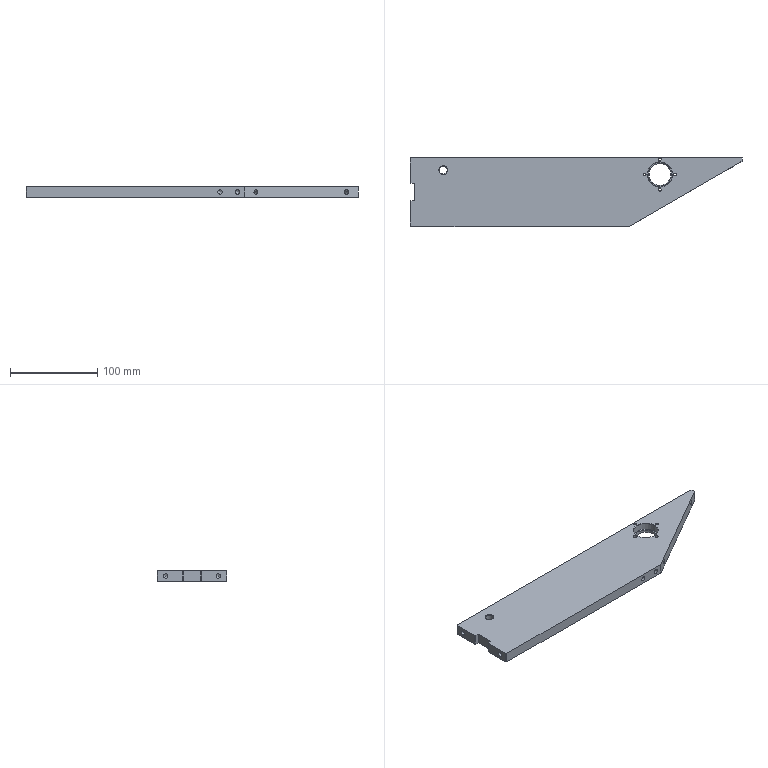Part | NX | 1 solid | 41 faces | box 380 x 80 x 12 mm | volume 295210 mm3 | plane 17 | cylinder 13 | cone 11 | commonest cylinder face diameters 5 x6 3.3 x4 9 x1 25 x1 28 x1
STEP:
#1=CARTESIAN_POINT('',(-190.,-32.5,-6.));
#2=VERTEX_POINT('',#1);
#3=CARTESIAN_POINT('',(-190.,-30.,-6.));
#4=DIRECTION('',(-1.,0.,0.));
#5=DIRECTION('',(0.,-1.,0.));
#6=AXIS2_PLACEMENT_3D('',#3,#4,#5);
#7=CIRCLE('',#6,2.5);
#8=EDGE_CURVE('',#2,#2,#7,.T.);
#9=ORIENTED_EDGE('',*,*,#8,.F.);
#10=EDGE_LOOP('',(#9));
#11=FACE_BOUND('',#10,.T.);
#12=CARTESIAN_POINT('',(-190.,-11.,0.));
#13=VERTEX_POINT('',#12);
#14=CARTESIAN_POINT('',(-190.,-39.,0.));
#15=VERTEX_POINT('',#14);
#16=CARTESIAN_POINT('',(-190.,40.,0.));
#17=DIRECTION('',(0.,-1.,0.));
#18=VECTOR('',#17,1000.);
#19=LINE('',#16,#18);
#20=EDGE_CURVE('',#13,#15,#19,.T.);
#21=ORIENTED_EDGE('',*,*,#20,.F.);
#22=CARTESIAN_POINT('',(-190.,-11.,-12.));
#23=VERTEX_POINT('',#22);
#24=CARTESIAN_POINT('',(-190.,-11.,0.));
#25=DIRECTION('',(0.,0.,-1.));
#26=VECTOR('',#25,1000.);
#27=LINE('',#24,#26);
#28=EDGE_CURVE('',#13,#23,#27,.T.);
#29=ORIENTED_EDGE('',*,*,#28,.T.);
#30=CARTESIAN_POINT('',(-190.,-39.,-12.));
#31=VERTEX_POINT('',#30);
#32=CARTESIAN_POINT('',(-190.,40.,-12.));
#33=DIRECTION('',(0.,-1.,0.));
#34=VECTOR('',#33,1000.);
#35=LINE('',#32,#34);
#36=EDGE_CURVE('',#23,#31,#35,.T.);
#37=ORIENTED_EDGE('',*,*,#36,.T.);
#38=CARTESIAN_POINT('',(-190.,-39.,0.));
#39=DIRECTION('',(0.,0.,1.));
#40=VECTOR('',#39,1000.);
#41=LINE('',#38,#40);
#42=EDGE_CURVE('',#31,#15,#41,.T.);
#43=ORIENTED_EDGE('',*,*,#42,.T.);
#44=EDGE_LOOP('',(#21,#29,#37,#43));
#45=FACE_BOUND('',#44,.T.);
#46=CARTESIAN_POINT('',(-190.,40.,0.));
#47=DIRECTION('',(1.,0.,0.));
#48=DIRECTION('',(0.,1.,0.));
#49=AXIS2_PLACEMENT_3D('',#46,#47,#48);
#50=PLANE('',#49);
#51=ADVANCED_FACE('',(#11,#45),#50,.F.);
#52=CARTESIAN_POINT('',(168.66,40.,-3.7));
#53=VERTEX_POINT('',#52);
#54=CARTESIAN_POINT('',(168.66,40.,-8.3));
#55=VERTEX_POINT('',#54);
#56=CARTESIAN_POINT('',(168.66,40.,-3.7));
#57=CARTESIAN_POINT('',(168.16,40.,-4.356));
#58=CARTESIAN_POINT('',(167.409,40.,-5.999));
#59=CARTESIAN_POINT('',(168.153,40.,-7.635));
#60=CARTESIAN_POINT('',(168.66,40.,-8.3));
#61=B_SPLINE_CURVE_WITH_KNOTS('',3,(#56,#57,#58,#59,#60),.UNSPECIFIED.,.F.,.F.,(4,1,4),(0.001159,0.003632,0.006106),.UNSPECIFIED.);
#62=EDGE_CURVE('',#53,#55,#61,.T.);
#63=ORIENTED_EDGE('',*,*,#62,.T.);
#64=CARTESIAN_POINT('',(169.793,40.,-6.));
#65=DIRECTION('',(0.,-1.,0.));
#66=DIRECTION('',(1.,0.,0.));
#67=AXIS2_PLACEMENT_3D('',#64,#65,#66);
#68=ELLIPSE('',#67,2.887,2.5);
#69=EDGE_CURVE('',#55,#53,#68,.T.);
#70=ORIENTED_EDGE('',*,*,#69,.T.);
#71=EDGE_LOOP('',(#63,#70));
#72=FACE_BOUND('',#71,.T.);
#73=CARTESIAN_POINT('',(189.,40.,0.));
#74=VERTEX_POINT('',#73);
#75=CARTESIAN_POINT('',(-189.,40.,0.));
#76=VERTEX_POINT('',#75);
#77=CARTESIAN_POINT('',(-190.,40.,0.));
#78=DIRECTION('',(-1.,0.,0.));
#79=VECTOR('',#78,1000.);
#80=LINE('',#77,#79);
#81=EDGE_CURVE('',#74,#76,#80,.T.);
#82=ORIENTED_EDGE('',*,*,#81,.F.);
#83=CARTESIAN_POINT('',(189.,40.,-12.));
#84=VERTEX_POINT('',#83);
#85=CARTESIAN_POINT('',(189.,40.,0.));
#86=DIRECTION('',(0.,0.,-1.));
#87=VECTOR('',#86,1000.);
#88=LINE('',#85,#87);
#89=EDGE_CURVE('',#74,#84,#88,.T.);
#90=ORIENTED_EDGE('',*,*,#89,.T.);
#91=CARTESIAN_POINT('',(-189.,40.,-12.));
#92=VERTEX_POINT('',#91);
#93=CARTESIAN_POINT('',(-190.,40.,-12.));
#94=DIRECTION('',(-1.,0.,0.));
#95=VECTOR('',#94,1000.);
#96=LINE('',#93,#95);
#97=EDGE_CURVE('',#84,#92,#96,.T.);
#98=ORIENTED_EDGE('',*,*,#97,.T.);
#99=CARTESIAN_POINT('',(-189.,40.,0.));
#100=DIRECTION('',(0.,0.,1.));
#101=VECTOR('',#100,1000.);
#102=LINE('',#99,#101);
#103=EDGE_CURVE('',#92,#76,#102,.T.);
#104=ORIENTED_EDGE('',*,*,#103,.T.);
#105=EDGE_LOOP('',(#82,#90,#98,#104));
#106=FACE_BOUND('',#105,.T.);
#107=CARTESIAN_POINT('',(-190.,40.,0.));
#108=DIRECTION('',(0.,-1.,0.));
#109=DIRECTION('',(0.,0.,-1.));
#110=AXIS2_PLACEMENT_3D('',#107,#108,#109);
#111=PLANE('',#110);
#112=ADVANCED_FACE('',(#72,#106),#111,.F.);
#113=CARTESIAN_POINT('',(-190.,27.5,-6.));
#114=VERTEX_POINT('',#113);
#115=CARTESIAN_POINT('',(-190.,30.,-6.));
#116=DIRECTION('',(-1.,0.,0.));
#117=DIRECTION('',(0.,-1.,0.));
#118=AXIS2_PLACEMENT_3D('',#115,#116,#117);
#119=CIRCLE('',#118,2.5);
#120=EDGE_CURVE('',#114,#114,#119,.T.);
#121=ORIENTED_EDGE('',*,*,#120,.F.);
#122=EDGE_LOOP('',(#121));
#123=FACE_BOUND('',#122,.T.);
#124=CARTESIAN_POINT('',(-190.,39.,-12.));
#125=VERTEX_POINT('',#124);
#126=CARTESIAN_POINT('',(-190.,11.,-12.));
#127=VERTEX_POINT('',#126);
#128=CARTESIAN_POINT('',(-190.,40.,-12.));
#129=DIRECTION('',(0.,-1.,0.));
#130=VECTOR('',#129,1000.);
#131=LINE('',#128,#130);
#132=EDGE_CURVE('',#125,#127,#131,.T.);
#133=ORIENTED_EDGE('',*,*,#132,.T.);
#134=CARTESIAN_POINT('',(-190.,11.,0.));
#135=VERTEX_POINT('',#134);
#136=CARTESIAN_POINT('',(-190.,11.,0.));
#137=DIRECTION('',(0.,0.,1.));
#138=VECTOR('',#137,1000.);
#139=LINE('',#136,#138);
#140=EDGE_CURVE('',#127,#135,#139,.T.);
#141=ORIENTED_EDGE('',*,*,#140,.T.);
#142=CARTESIAN_POINT('',(-190.,39.,0.));
#143=VERTEX_POINT('',#142);
#144=CARTESIAN_POINT('',(-190.,40.,0.));
#145=DIRECTION('',(0.,-1.,0.));
#146=VECTOR('',#145,1000.);
#147=LINE('',#144,#146);
#148=EDGE_CURVE('',#143,#135,#147,.T.);
#149=ORIENTED_EDGE('',*,*,#148,.F.);
#150=CARTESIAN_POINT('',(-190.,39.,0.));
#151=DIRECTION('',(0.,0.,-1.));
#152=VECTOR('',#151,1000.);
#153=LINE('',#150,#152);
#154=EDGE_CURVE('',#143,#125,#153,.T.);
#155=ORIENTED_EDGE('',*,*,#154,.T.);
#156=EDGE_LOOP('',(#133,#141,#149,#155));
#157=FACE_BOUND('',#156,.T.);
#158=CARTESIAN_POINT('',(-190.,40.,0.));
#159=DIRECTION('',(1.,0.,0.));
#160=DIRECTION('',(0.,1.,0.));
#161=AXIS2_PLACEMENT_3D('',#158,#159,#160);
#162=PLANE('',#161);
#163=ADVANCED_FACE('',(#123,#157),#162,.F.);
#164=CARTESIAN_POINT('',(52.096,-40.,-8.5));
#165=VERTEX_POINT('',#164);
#166=CARTESIAN_POINT('',(52.096,-40.,-6.));
#167=DIRECTION('',(0.,-1.,0.));
#168=DIRECTION('',(0.,0.,-1.));
#169=AXIS2_PLACEMENT_3D('',#166,#167,#168);
#170=CIRCLE('',#169,2.5);
#171=EDGE_CURVE('',#165,#165,#170,.T.);
#172=ORIENTED_EDGE('',*,*,#171,.F.);
#173=EDGE_LOOP('',(#172));
#174=FACE_BOUND('',#173,.T.);
#175=CARTESIAN_POINT('',(32.096,-40.,-8.5));
#176=VERTEX_POINT('',#175);
#177=CARTESIAN_POINT('',(32.096,-40.,-6.));
#178=DIRECTION('',(0.,-1.,0.));
#179=DIRECTION('',(0.,0.,-1.));
#180=AXIS2_PLACEMENT_3D('',#177,#178,#179);
#181=CIRCLE('',#180,2.5);
#182=EDGE_CURVE('',#176,#176,#181,.T.);
#183=ORIENTED_EDGE('',*,*,#182,.F.);
#184=EDGE_LOOP('',(#183));
#185=FACE_BOUND('',#184,.T.);
#186=CARTESIAN_POINT('',(-189.,-40.,0.));
#187=VERTEX_POINT('',#186);
#188=CARTESIAN_POINT('',(60.096,-40.,0.));
#189=VERTEX_POINT('',#188);
#190=CARTESIAN_POINT('',(-190.,-40.,0.));
#191=DIRECTION('',(1.,0.,0.));
#192=VECTOR('',#191,1000.);
#193=LINE('',#190,#192);
#194=EDGE_CURVE('',#187,#189,#193,.T.);
#195=ORIENTED_EDGE('',*,*,#194,.F.);
#196=CARTESIAN_POINT('',(-189.,-40.,-12.));
#197=VERTEX_POINT('',#196);
#198=CARTESIAN_POINT('',(-189.,-40.,0.));
#199=DIRECTION('',(0.,0.,-1.));
#200=VECTOR('',#199,1000.);
#201=LINE('',#198,#200);
#202=EDGE_CURVE('',#187,#197,#201,.T.);
#203=ORIENTED_EDGE('',*,*,#202,.T.);
#204=CARTESIAN_POINT('',(60.096,-40.,-12.));
#205=VERTEX_POINT('',#204);
#206=CARTESIAN_POINT('',(-190.,-40.,-12.));
#207=DIRECTION('',(1.,0.,0.));
#208=VECTOR('',#207,1000.);
#209=LINE('',#206,#208);
#210=EDGE_CURVE('',#197,#205,#209,.T.);
#211=ORIENTED_EDGE('',*,*,#210,.T.);
#212=CARTESIAN_POINT('',(60.096,-40.,0.));
#213=DIRECTION('',(0.,0.,-1.));
#214=VECTOR('',#213,1000.);
#215=LINE('',#212,#214);
#216=EDGE_CURVE('',#189,#205,#215,.T.);
#217=ORIENTED_EDGE('',*,*,#216,.F.);
#218=EDGE_LOOP('',(#195,#203,#211,#217));
#219=FACE_BOUND('',#218,.T.);
#220=CARTESIAN_POINT('',(-190.,-40.,0.));
#221=DIRECTION('',(0.,1.,0.));
#222=DIRECTION('',(0.,0.,1.));
#223=AXIS2_PLACEMENT_3D('',#220,#221,#222);
#224=PLANE('',#223);
#225=ADVANCED_FACE('',(#174,#185,#219),#224,.F.);
#226=CARTESIAN_POINT('',(179.175,28.75,-6.));
#227=VERTEX_POINT('',#226);
#228=CARTESIAN_POINT('',(177.01,27.5,-6.));
#229=DIRECTION('',(0.5,-0.866,0.));
#230=DIRECTION('',(0.866,0.5,0.));
#231=AXIS2_PLACEMENT_3D('',#228,#229,#230);
#232=CIRCLE('',#231,2.5);
#233=EDGE_CURVE('',#227,#227,#232,.T.);
#234=ORIENTED_EDGE('',*,*,#233,.F.);
#235=EDGE_LOOP('',(#234));
#236=FACE_BOUND('',#235,.T.);
#237=CARTESIAN_POINT('',(75.252,-31.25,-6.));
#238=VERTEX_POINT('',#237);
#239=CARTESIAN_POINT('',(73.087,-32.5,-6.));
#240=DIRECTION('',(0.5,-0.866,0.));
#241=DIRECTION('',(0.866,0.5,0.));
#242=AXIS2_PLACEMENT_3D('',#239,#240,#241);
#243=CIRCLE('',#242,2.5);
#244=EDGE_CURVE('',#238,#238,#243,.T.);
#245=ORIENTED_EDGE('',*,*,#244,.F.);
#246=EDGE_LOOP('',(#245));
#247=FACE_BOUND('',#246,.T.);
#248=CARTESIAN_POINT('',(190.,35.,-12.));
#249=VERTEX_POINT('',#248);
#250=CARTESIAN_POINT('',(190.,35.,-12.));
#251=DIRECTION('',(0.866,0.5,0.));
#252=VECTOR('',#251,1000.);
#253=LINE('',#250,#252);
#254=EDGE_CURVE('',#205,#249,#253,.T.);
#255=ORIENTED_EDGE('',*,*,#254,.T.);
#256=CARTESIAN_POINT('',(190.,35.,0.));
#257=VERTEX_POINT('',#256);
#258=CARTESIAN_POINT('',(190.,35.,0.));
#259=DIRECTION('',(0.,0.,-1.));
#260=VECTOR('',#259,1000.);
#261=LINE('',#258,#260);
#262=EDGE_CURVE('',#257,#249,#261,.T.);
#263=ORIENTED_EDGE('',*,*,#262,.F.);
#264=CARTESIAN_POINT('',(190.,35.,0.));
#265=DIRECTION('',(0.866,0.5,0.));
#266=VECTOR('',#265,1000.);
#267=LINE('',#264,#266);
#268=EDGE_CURVE('',#189,#257,#267,.T.);
#269=ORIENTED_EDGE('',*,*,#268,.F.);
#270=ORIENTED_EDGE('',*,*,#216,.T.);
#271=EDGE_LOOP('',(#255,#263,#269,#270));
#272=FACE_BOUND('',#271,.T.);
#273=CARTESIAN_POINT('',(190.,35.,0.));
#274=DIRECTION('',(-0.5,0.866,0.));
#275=DIRECTION('',(-0.866,-0.5,0.));
#276=AXIS2_PLACEMENT_3D('',#273,#274,#275);
#277=PLANE('',#276);
#278=ADVANCED_FACE('',(#236,#247,#272),#277,.F.);
#279=CARTESIAN_POINT('',(190.,39.,-12.));
#280=VERTEX_POINT('',#279);
#281=CARTESIAN_POINT('',(190.,40.,-12.));
#282=DIRECTION('',(0.,1.,0.));
#283=VECTOR('',#282,1000.);
#284=LINE('',#281,#283);
#285=EDGE_CURVE('',#249,#280,#284,.T.);
#286=ORIENTED_EDGE('',*,*,#285,.T.);
#287=CARTESIAN_POINT('',(190.,39.,0.));
#288=VERTEX_POINT('',#287);
#289=CARTESIAN_POINT('',(190.,39.,0.));
#290=DIRECTION('',(0.,0.,1.));
#291=VECTOR('',#290,1000.);
#292=LINE('',#289,#291);
#293=EDGE_CURVE('',#280,#288,#292,.T.);
#294=ORIENTED_EDGE('',*,*,#293,.T.);
#295=CARTESIAN_POINT('',(190.,40.,0.));
#296=DIRECTION('',(0.,1.,0.));
#297=VECTOR('',#296,1000.);
#298=LINE('',#295,#297);
#299=EDGE_CURVE('',#257,#288,#298,.T.);
#300=ORIENTED_EDGE('',*,*,#299,.F.);
#301=ORIENTED_EDGE('',*,*,#262,.T.);
#302=EDGE_LOOP('',(#286,#294,#300,#301));
#303=FACE_BOUND('',#302,.T.);
#304=CARTESIAN_POINT('',(190.,40.,0.));
#305=DIRECTION('',(-1.,0.,0.));
#306=DIRECTION('',(0.,-1.,0.));
#307=AXIS2_PLACEMENT_3D('',#304,#305,#306);
#308=PLANE('',#307);
#309=ADVANCED_FACE('',(#303),#308,.F.);
#310=CARTESIAN_POINT('',(-152.,30.,0.));
#311=VERTEX_POINT('',#310);
#312=CARTESIAN_POINT('',(-152.,25.,0.));
#313=DIRECTION('',(0.,0.,-1.));
#314=DIRECTION('',(0.,1.,0.));
#315=AXIS2_PLACEMENT_3D('',#312,#313,#314);
#316=CIRCLE('',#315,5.);
#317=EDGE_CURVE('',#311,#311,#316,.T.);
#318=ORIENTED_EDGE('',*,*,#317,.T.);
#319=EDGE_LOOP('',(#318));
#320=FACE_BOUND('',#319,.T.);
#321=CARTESIAN_POINT('',(96.,34.5,0.));
#322=VERTEX_POINT('',#321);
#323=CARTESIAN_POINT('',(96.,20.,0.));
#324=DIRECTION('',(0.,0.,-1.));
#325=DIRECTION('',(0.,1.,0.));
#326=AXIS2_PLACEMENT_3D('',#323,#324,#325);
#327=CIRCLE('',#326,14.5);
#328=EDGE_CURVE('',#322,#322,#327,.T.);
#329=ORIENTED_EDGE('',*,*,#328,.T.);
#330=EDGE_LOOP('',(#329));
#331=FACE_BOUND('',#330,.T.);
#332=CARTESIAN_POINT('',(94.35,37.5,0.));
#333=VERTEX_POINT('',#332);
#334=CARTESIAN_POINT('',(96.,37.5,0.));
#335=DIRECTION('',(0.,0.,-1.));
#336=DIRECTION('',(-1.,0.,0.));
#337=AXIS2_PLACEMENT_3D('',#334,#335,#336);
#338=CIRCLE('',#337,1.65);
#339=EDGE_CURVE('',#333,#333,#338,.T.);
#340=ORIENTED_EDGE('',*,*,#339,.T.);
#341=EDGE_LOOP('',(#340));
#342=FACE_BOUND('',#341,.T.);
#343=CARTESIAN_POINT('',(78.5,18.35,0.));
#344=VERTEX_POINT('',#343);
#345=CARTESIAN_POINT('',(78.5,20.,0.));
#346=DIRECTION('',(0.,0.,-1.));
#347=DIRECTION('',(0.,-1.,0.));
#348=AXIS2_PLACEMENT_3D('',#345,#346,#347);
#349=CIRCLE('',#348,1.65);
#350=EDGE_CURVE('',#344,#344,#349,.T.);
#351=ORIENTED_EDGE('',*,*,#350,.T.);
#352=EDGE_LOOP('',(#351));
#353=FACE_BOUND('',#352,.T.);
#354=CARTESIAN_POINT('',(97.65,2.5,0.));
#355=VERTEX_POINT('',#354);
#356=CARTESIAN_POINT('',(96.,2.5,0.));
#357=DIRECTION('',(0.,0.,-1.));
#358=DIRECTION('',(1.,0.,0.));
#359=AXIS2_PLACEMENT_3D('',#356,#357,#358);
#360=CIRCLE('',#359,1.65);
#361=EDGE_CURVE('',#355,#355,#360,.T.);
#362=ORIENTED_EDGE('',*,*,#361,.T.);
#363=EDGE_LOOP('',(#362));
#364=FACE_BOUND('',#363,.T.);
#365=CARTESIAN_POINT('',(113.5,21.65,0.));
#366=VERTEX_POINT('',#365);
#367=CARTESIAN_POINT('',(113.5,20.,0.));
#368=DIRECTION('',(0.,0.,-1.));
#369=DIRECTION('',(0.,1.,0.));
#370=AXIS2_PLACEMENT_3D('',#367,#368,#369);
#371=CIRCLE('',#370,1.65);
#372=EDGE_CURVE('',#366,#366,#371,.T.);
#373=ORIENTED_EDGE('',*,*,#372,.T.);
#374=EDGE_LOOP('',(#373));
#375=FACE_BOUND('',#374,.T.);
#376=CARTESIAN_POINT('',(-189.,-10.,0.));
#377=VERTEX_POINT('',#376);
#378=CARTESIAN_POINT('',(-185.,-10.,0.));
#379=VERTEX_POINT('',#378);
#380=CARTESIAN_POINT('',(-195.,-10.,0.));
#381=DIRECTION('',(1.,0.,0.));
#382=VECTOR('',#381,1000.);
#383=LINE('',#380,#382);
#384=EDGE_CURVE('',#377,#379,#383,.T.);
#385=ORIENTED_EDGE('',*,*,#384,.F.);
#386=CARTESIAN_POINT('',(-190.,-11.,0.));
#387=DIRECTION('',(0.7071,0.7071,0.));
#388=VECTOR('',#387,1000.);
#389=LINE('',#386,#388);
#390=EDGE_CURVE('',#377,#13,#389,.F.);
#391=ORIENTED_EDGE('',*,*,#390,.T.);
#392=ORIENTED_EDGE('',*,*,#20,.T.);
#393=CARTESIAN_POINT('',(-189.,-40.,0.));
#394=DIRECTION('',(-0.7071,0.7071,0.));
#395=VECTOR('',#394,1000.);
#396=LINE('',#393,#395);
#397=EDGE_CURVE('',#15,#187,#396,.F.);
#398=ORIENTED_EDGE('',*,*,#397,.T.);
#399=ORIENTED_EDGE('',*,*,#194,.T.);
#400=ORIENTED_EDGE('',*,*,#268,.T.);
#401=ORIENTED_EDGE('',*,*,#299,.T.);
#402=CARTESIAN_POINT('',(189.,40.,0.));
#403=DIRECTION('',(0.7071,-0.7071,0.));
#404=VECTOR('',#403,1000.);
#405=LINE('',#402,#404);
#406=EDGE_CURVE('',#288,#74,#405,.F.);
#407=ORIENTED_EDGE('',*,*,#406,.T.);
#408=ORIENTED_EDGE('',*,*,#81,.T.);
#409=CARTESIAN_POINT('',(-190.,39.,0.));
#410=DIRECTION('',(0.7071,0.7071,0.));
#411=VECTOR('',#410,1000.);
#412=LINE('',#409,#411);
#413=EDGE_CURVE('',#76,#143,#412,.F.);
#414=ORIENTED_EDGE('',*,*,#413,.T.);
#415=ORIENTED_EDGE('',*,*,#148,.T.);
#416=CARTESIAN_POINT('',(-189.,10.,0.));
#417=VERTEX_POINT('',#416);
#418=CARTESIAN_POINT('',(-190.,11.,0.));
#419=DIRECTION('',(-0.7071,0.7071,0.));
#420=VECTOR('',#419,1000.);
#421=LINE('',#418,#420);
#422=EDGE_CURVE('',#135,#417,#421,.F.);
#423=ORIENTED_EDGE('',*,*,#422,.T.);
#424=CARTESIAN_POINT('',(-185.,10.,0.));
#425=VERTEX_POINT('',#424);
#426=CARTESIAN_POINT('',(-195.,10.,0.));
#427=DIRECTION('',(-1.,0.,0.));
#428=VECTOR('',#427,1000.);
#429=LINE('',#426,#428);
#430=EDGE_CURVE('',#425,#417,#429,.T.);
#431=ORIENTED_EDGE('',*,*,#430,.F.);
#432=CARTESIAN_POINT('',(-185.,10.,0.));
#433=DIRECTION('',(0.,1.,0.));
#434=VECTOR('',#433,1000.);
#435=LINE('',#432,#434);
#436=EDGE_CURVE('',#379,#425,#435,.T.);
#437=ORIENTED_EDGE('',*,*,#436,.F.);
#438=EDGE_LOOP('',(#385,#391,#392,#398,#399,#400,#401,#407,#408,#414,#415,#423,#431,#437));
#439=FACE_BOUND('',#438,.T.);
#440=CARTESIAN_POINT('',(-190.,40.,0.));
#441=DIRECTION('',(0.,0.,-1.));
#442=DIRECTION('',(0.,1.,0.));
#443=AXIS2_PLACEMENT_3D('',#440,#441,#442);
#444=PLANE('',#443);
#445=ADVANCED_FACE('',(#320,#331,#342,#353,#364,#375,#439),#444,.F.);
#446=CARTESIAN_POINT('',(-152.,30.,-12.));
#447=VERTEX_POINT('',#446);
#448=CARTESIAN_POINT('',(-152.,25.,-12.));
#449=DIRECTION('',(0.,0.,-1.));
#450=DIRECTION('',(0.,1.,0.));
#451=AXIS2_PLACEMENT_3D('',#448,#449,#450);
#452=CIRCLE('',#451,5.);
#453=EDGE_CURVE('',#447,#447,#452,.F.);
#454=ORIENTED_EDGE('',*,*,#453,.T.);
#455=EDGE_LOOP('',(#454));
#456=FACE_BOUND('',#455,.T.);
#457=ORIENTED_EDGE('',*,*,#36,.F.);
#458=CARTESIAN_POINT('',(-189.,-10.,-12.));
#459=VERTEX_POINT('',#458);
#460=CARTESIAN_POINT('',(-164.5,14.5,-12.));
#461=DIRECTION('',(-0.7071,-0.7071,0.));
#462=VECTOR('',#461,1000.);
#463=LINE('',#460,#462);
#464=EDGE_CURVE('',#23,#459,#463,.F.);
#465=ORIENTED_EDGE('',*,*,#464,.T.);
#466=CARTESIAN_POINT('',(-185.,-10.,-12.));
#467=VERTEX_POINT('',#466);
#468=CARTESIAN_POINT('',(-190.,-10.,-12.));
#469=DIRECTION('',(-1.,0.,0.));
#470=VECTOR('',#469,1000.);
#471=LINE('',#468,#470);
#472=EDGE_CURVE('',#467,#459,#471,.T.);
#473=ORIENTED_EDGE('',*,*,#472,.F.);
#474=CARTESIAN_POINT('',(-185.,10.,-12.));
#475=VERTEX_POINT('',#474);
#476=CARTESIAN_POINT('',(-185.,10.,-12.));
#477=DIRECTION('',(0.,1.,0.));
#478=VECTOR('',#477,1000.);
#479=LINE('',#476,#478);
#480=EDGE_CURVE('',#467,#475,#479,.T.);
#481=ORIENTED_EDGE('',*,*,#480,.T.);
#482=CARTESIAN_POINT('',(-189.,10.,-12.));
#483=VERTEX_POINT('',#482);
#484=CARTESIAN_POINT('',(-195.,10.,-12.));
#485=DIRECTION('',(-1.,0.,0.));
#486=VECTOR('',#485,1000.);
#487=LINE('',#484,#486);
#488=EDGE_CURVE('',#475,#483,#487,.T.);
#489=ORIENTED_EDGE('',*,*,#488,.T.);
#490=CARTESIAN_POINT('',(-204.5,25.5,-12.));
#491=DIRECTION('',(0.7071,-0.7071,0.));
#492=VECTOR('',#491,1000.);
#493=LINE('',#490,#492);
#494=EDGE_CURVE('',#483,#127,#493,.F.);
#495=ORIENTED_EDGE('',*,*,#494,.T.);
#496=ORIENTED_EDGE('',*,*,#132,.F.);
#497=CARTESIAN_POINT('',(-189.5,39.5,-12.));
#498=DIRECTION('',(-0.7071,-0.7071,0.));
#499=VECTOR('',#498,1000.);
#500=LINE('',#497,#499);
#501=EDGE_CURVE('',#125,#92,#500,.F.);
#502=ORIENTED_EDGE('',*,*,#501,.T.);
#503=ORIENTED_EDGE('',*,*,#97,.F.);
#504=CARTESIAN_POINT('',(-0.5,229.5,-12.));
#505=DIRECTION('',(-0.7071,0.7071,0.));
#506=VECTOR('',#505,1000.);
#507=LINE('',#504,#506);
#508=EDGE_CURVE('',#84,#280,#507,.F.);
#509=ORIENTED_EDGE('',*,*,#508,.T.);
#510=ORIENTED_EDGE('',*,*,#285,.F.);
#511=ORIENTED_EDGE('',*,*,#254,.F.);
#512=ORIENTED_EDGE('',*,*,#210,.F.);
#513=CARTESIAN_POINT('',(-229.5,0.5,-12.));
#514=DIRECTION('',(0.7071,-0.7071,0.));
#515=VECTOR('',#514,1000.);
#516=LINE('',#513,#515);
#517=EDGE_CURVE('',#197,#31,#516,.F.);
#518=ORIENTED_EDGE('',*,*,#517,.T.);
#519=EDGE_LOOP('',(#457,#465,#473,#481,#489,#495,#496,#502,#503,#509,#510,#511,#512,#518));
#520=FACE_BOUND('',#519,.T.);
#521=CARTESIAN_POINT('',(96.,33.,-12.));
#522=VERTEX_POINT('',#521);
#523=CARTESIAN_POINT('',(96.,20.,-12.));
#524=DIRECTION('',(0.,0.,-1.));
#525=DIRECTION('',(0.,1.,0.));
#526=AXIS2_PLACEMENT_3D('',#523,#524,#525);
#527=CIRCLE('',#526,13.);
#528=EDGE_CURVE('',#522,#522,#527,.F.);
#529=ORIENTED_EDGE('',*,*,#528,.T.);
#530=EDGE_LOOP('',(#529));
#531=FACE_BOUND('',#530,.T.);
#532=CARTESIAN_POINT('',(94.35,37.5,-12.));
#533=VERTEX_POINT('',#532);
#534=CARTESIAN_POINT('',(96.,37.5,-12.));
#535=DIRECTION('',(0.,0.,-1.));
#536=DIRECTION('',(-1.,0.,0.));
#537=AXIS2_PLACEMENT_3D('',#534,#535,#536);
#538=CIRCLE('',#537,1.65);
#539=EDGE_CURVE('',#533,#533,#538,.T.);
#540=ORIENTED_EDGE('',*,*,#539,.F.);
#541=EDGE_LOOP('',(#540));
#542=FACE_BOUND('',#541,.T.);
#543=CARTESIAN_POINT('',(78.5,18.35,-12.));
#544=VERTEX_POINT('',#543);
#545=CARTESIAN_POINT('',(78.5,20.,-12.));
#546=DIRECTION('',(0.,0.,-1.));
#547=DIRECTION('',(0.,-1.,0.));
#548=AXIS2_PLACEMENT_3D('',#545,#546,#547);
#549=CIRCLE('',#548,1.65);
#550=EDGE_CURVE('',#544,#544,#549,.T.);
#551=ORIENTED_EDGE('',*,*,#550,.F.);
#552=EDGE_LOOP('',(#551));
#553=FACE_BOUND('',#552,.T.);
#554=CARTESIAN_POINT('',(97.65,2.5,-12.));
#555=VERTEX_POINT('',#554);
#556=CARTESIAN_POINT('',(96.,2.5,-12.));
#557=DIRECTION('',(0.,0.,-1.));
#558=DIRECTION('',(1.,0.,0.));
#559=AXIS2_PLACEMENT_3D('',#556,#557,#558);
#560=CIRCLE('',#559,1.65);
#561=EDGE_CURVE('',#555,#555,#560,.T.);
#562=ORIENTED_EDGE('',*,*,#561,.F.);
#563=EDGE_LOOP('',(#562));
#564=FACE_BOUND('',#563,.T.);
#565=CARTESIAN_POINT('',(113.5,21.65,-12.));
#566=VERTEX_POINT('',#565);
#567=CARTESIAN_POINT('',(113.5,20.,-12.));
#568=DIRECTION('',(0.,0.,-1.));
#569=DIRECTION('',(0.,1.,0.));
#570=AXIS2_PLACEMENT_3D('',#567,#568,#569);
#571=CIRCLE('',#570,1.65);
#572=EDGE_CURVE('',#566,#566,#571,.T.);
#573=ORIENTED_EDGE('',*,*,#572,.F.);
#574=EDGE_LOOP('',(#573));
#575=FACE_BOUND('',#574,.T.);
#576=CARTESIAN_POINT('',(-190.,40.,-12.));
#577=DIRECTION('',(0.,0.,-1.));
#578=DIRECTION('',(0.,1.,0.));
#579=AXIS2_PLACEMENT_3D('',#576,#577,#578);
#580=PLANE('',#579);
#581=ADVANCED_FACE('',(#456,#520,#531,#542,#553,#564,#575),#580,.T.);
#582=CARTESIAN_POINT('',(64.865,-18.26,-6.));
#583=VERTEX_POINT('',#582);
#584=VERTEX_LOOP('',#583);
#585=FACE_BOUND('',#584,.T.);
#586=CARTESIAN_POINT('',(67.752,-18.26,-6.));
#587=VERTEX_POINT('',#586);
#588=CARTESIAN_POINT('',(65.587,-19.51,-6.));
#589=DIRECTION('',(0.5,-0.866,0.));
#590=DIRECTION('',(0.866,0.5,0.));
#591=AXIS2_PLACEMENT_3D('',#588,#589,#590);
#592=CIRCLE('',#591,2.5);
#593=EDGE_CURVE('',#587,#587,#592,.T.);
#594=ORIENTED_EDGE('',*,*,#593,.T.);
#595=EDGE_LOOP('',(#594));
#596=FACE_BOUND('',#595,.T.);
#597=CARTESIAN_POINT('',(65.587,-19.51,-6.));
#598=DIRECTION('',(0.5,-0.866,0.));
#599=DIRECTION('',(0.866,0.5,0.));
#600=AXIS2_PLACEMENT_3D('',#597,#598,#599);
#601=CONICAL_SURFACE('',#600,2.5,1.047);
#602=ADVANCED_FACE('',(#585,#596),#601,.F.);
#603=ORIENTED_EDGE('',*,*,#593,.F.);
#604=EDGE_LOOP('',(#603));
#605=FACE_BOUND('',#604,.T.);
#606=ORIENTED_EDGE('',*,*,#244,.T.);
#607=EDGE_LOOP('',(#606));
#608=FACE_BOUND('',#607,.T.);
#609=CARTESIAN_POINT('',(73.087,-32.5,-6.));
#610=DIRECTION('',(0.5,-0.866,0.));
#611=DIRECTION('',(0.866,0.5,0.));
#612=AXIS2_PLACEMENT_3D('',#609,#610,#611);
#613=CYLINDRICAL_SURFACE('',#612,2.5);
#614=ADVANCED_FACE('',(#605,#608),#613,.F.);
#615=ORIENTED_EDGE('',*,*,#233,.T.);
#616=EDGE_LOOP('',(#615));
#617=FACE_BOUND('',#616,.T.);
#618=CARTESIAN_POINT('',(169.51,40.49,-6.));
#619=DIRECTION('',(0.5,-0.866,0.));
#620=DIRECTION('',(0.866,0.5,0.));
#621=AXIS2_PLACEMENT_3D('',#618,#619,#620);
#622=CIRCLE('',#621,2.5);
#623=EDGE_CURVE('',#53,#55,#622,.T.);
#624=ORIENTED_EDGE('',*,*,#623,.F.);
#625=ORIENTED_EDGE('',*,*,#69,.F.);
#626=EDGE_LOOP('',(#624,#625));
#627=FACE_BOUND('',#626,.T.);
#628=CARTESIAN_POINT('',(177.01,27.5,-6.));
#629=DIRECTION('',(0.5,-0.866,0.));
#630=DIRECTION('',(0.866,0.5,0.));
#631=AXIS2_PLACEMENT_3D('',#628,#629,#630);
#632=CYLINDRICAL_SURFACE('',#631,2.5);
#633=ADVANCED_FACE('',(#617,#627),#632,.F.);
#634=ORIENTED_EDGE('',*,*,#623,.T.);
#635=ORIENTED_EDGE('',*,*,#62,.F.);
#636=EDGE_LOOP('',(#634,#635));
#637=FACE_BOUND('',#636,.T.);
#638=CARTESIAN_POINT('',(169.51,40.49,-6.));
#639=DIRECTION('',(0.5,-0.866,0.));
#640=DIRECTION('',(0.866,0.5,0.));
#641=AXIS2_PLACEMENT_3D('',#638,#639,#640);
#642=CONICAL_SURFACE('',#641,2.5,1.047);
#643=ADVANCED_FACE('',(#637),#642,.F.);
#644=ORIENTED_EDGE('',*,*,#406,.F.);
#645=ORIENTED_EDGE('',*,*,#293,.F.);
#646=ORIENTED_EDGE('',*,*,#508,.F.);
#647=ORIENTED_EDGE('',*,*,#89,.F.);
#648=EDGE_LOOP('',(#644,#645,#646,#647));
#649=FACE_BOUND('',#648,.T.);
#650=CARTESIAN_POINT('',(189.,40.,0.));
#651=DIRECTION('',(-0.7071,-0.7071,0.));
#652=DIRECTION('',(0.,0.,-1.));
#653=AXIS2_PLACEMENT_3D('',#650,#651,#652);
#654=PLANE('',#653);
#655=ADVANCED_FACE('',(#649),#654,.F.);
#656=ORIENTED_EDGE('',*,*,#413,.F.);
#657=ORIENTED_EDGE('',*,*,#103,.F.);
#658=ORIENTED_EDGE('',*,*,#501,.F.);
#659=ORIENTED_EDGE('',*,*,#154,.F.);
#660=EDGE_LOOP('',(#656,#657,#658,#659));
#661=FACE_BOUND('',#660,.T.);
#662=CARTESIAN_POINT('',(-190.,39.,0.));
#663=DIRECTION('',(0.7071,-0.7071,0.));
#664=DIRECTION('',(0.,0.,-1.));
#665=AXIS2_PLACEMENT_3D('',#662,#663,#664);
#666=PLANE('',#665);
#667=ADVANCED_FACE('',(#661),#666,.F.);
#668=ORIENTED_EDGE('',*,*,#397,.F.);
#669=ORIENTED_EDGE('',*,*,#42,.F.);
#670=ORIENTED_EDGE('',*,*,#517,.F.);
#671=ORIENTED_EDGE('',*,*,#202,.F.);
#672=EDGE_LOOP('',(#668,#669,#670,#671));
#673=FACE_BOUND('',#672,.T.);
#674=CARTESIAN_POINT('',(-189.,-40.,0.));
#675=DIRECTION('',(0.7071,0.7071,0.));
#676=DIRECTION('',(0.,0.,-1.));
#677=AXIS2_PLACEMENT_3D('',#674,#675,#676);
#678=PLANE('',#677);
#679=ADVANCED_FACE('',(#673),#678,.F.);
#680=CARTESIAN_POINT('',(96.,32.5,-11.5));
#681=VERTEX_POINT('',#680);
#682=CARTESIAN_POINT('',(96.,20.,-11.5));
#683=DIRECTION('',(0.,0.,-1.));
#684=DIRECTION('',(0.,1.,0.));
#685=AXIS2_PLACEMENT_3D('',#682,#683,#684);
#686=CIRCLE('',#685,12.5);
#687=EDGE_CURVE('',#681,#681,#686,.T.);
#688=ORIENTED_EDGE('',*,*,#687,.T.);
#689=EDGE_LOOP('',(#688));
#690=FACE_BOUND('',#689,.T.);
#691=CARTESIAN_POINT('',(96.,32.5,-8.5));
#692=VERTEX_POINT('',#691);
#693=CARTESIAN_POINT('',(96.,20.,-8.5));
#694=DIRECTION('',(0.,0.,-1.));
#695=DIRECTION('',(0.,1.,0.));
#696=AXIS2_PLACEMENT_3D('',#693,#694,#695);
#697=CIRCLE('',#696,12.5);
#698=EDGE_CURVE('',#692,#692,#697,.F.);
#699=ORIENTED_EDGE('',*,*,#698,.T.);
#700=EDGE_LOOP('',(#699));
#701=FACE_BOUND('',#700,.T.);
#702=CARTESIAN_POINT('',(96.,20.,-12.));
#703=DIRECTION('',(0.,0.,1.));
#704=DIRECTION('',(0.,-1.,0.));
#705=AXIS2_PLACEMENT_3D('',#702,#703,#704);
#706=CYLINDRICAL_SURFACE('',#705,12.5);
#707=ADVANCED_FACE('',(#690,#701),#706,.F.);
#708=CARTESIAN_POINT('',(96.,33.,-8.));
#709=VERTEX_POINT('',#708);
#710=CARTESIAN_POINT('',(96.,20.,-8.));
#711=DIRECTION('',(0.,0.,-1.));
#712=DIRECTION('',(0.,1.,0.));
#713=AXIS2_PLACEMENT_3D('',#710,#711,#712);
#714=CIRCLE('',#713,13.);
#715=EDGE_CURVE('',#709,#709,#714,.T.);
#716=ORIENTED_EDGE('',*,*,#715,.T.);
#717=EDGE_LOOP('',(#716));
#718=FACE_BOUND('',#717,.T.);
#719=CARTESIAN_POINT('',(96.,34.,-8.));
#720=VERTEX_POINT('',#719);
#721=CARTESIAN_POINT('',(96.,20.,-8.));
#722=DIRECTION('',(0.,0.,-1.));
#723=DIRECTION('',(0.,1.,0.));
#724=AXIS2_PLACEMENT_3D('',#721,#722,#723);
#725=CIRCLE('',#724,14.);
#726=EDGE_CURVE('',#720,#720,#725,.T.);
#727=ORIENTED_EDGE('',*,*,#726,.F.);
#728=EDGE_LOOP('',(#727));
#729=FACE_BOUND('',#728,.T.);
#730=CARTESIAN_POINT('',(96.,20.,-8.));
#731=DIRECTION('',(0.,0.,-1.));
#732=DIRECTION('',(0.,1.,0.));
#733=AXIS2_PLACEMENT_3D('',#730,#731,#732);
#734=PLANE('',#733);
#735=ADVANCED_FACE('',(#718,#729),#734,.F.);
#736=CARTESIAN_POINT('',(96.,34.,-0.5));
#737=VERTEX_POINT('',#736);
#738=CARTESIAN_POINT('',(96.,20.,-0.5));
#739=DIRECTION('',(0.,0.,-1.));
#740=DIRECTION('',(0.,1.,0.));
#741=AXIS2_PLACEMENT_3D('',#738,#739,#740);
#742=CIRCLE('',#741,14.);
#743=EDGE_CURVE('',#737,#737,#742,.F.);
#744=ORIENTED_EDGE('',*,*,#743,.T.);
#745=EDGE_LOOP('',(#744));
#746=FACE_BOUND('',#745,.T.);
#747=ORIENTED_EDGE('',*,*,#726,.T.);
#748=EDGE_LOOP('',(#747));
#749=FACE_BOUND('',#748,.T.);
#750=CARTESIAN_POINT('',(96.,20.,-8.));
#751=DIRECTION('',(0.,0.,1.));
#752=DIRECTION('',(0.,-1.,0.));
#753=AXIS2_PLACEMENT_3D('',#750,#751,#752);
#754=CYLINDRICAL_SURFACE('',#753,14.);
#755=ADVANCED_FACE('',(#746,#749),#754,.F.);
#756=ORIENTED_EDGE('',*,*,#372,.F.);
#757=EDGE_LOOP('',(#756));
#758=FACE_BOUND('',#757,.T.);
#759=ORIENTED_EDGE('',*,*,#572,.T.);
#760=EDGE_LOOP('',(#759));
#761=FACE_BOUND('',#760,.T.);
#762=CARTESIAN_POINT('',(113.5,20.,-12.));
#763=DIRECTION('',(0.,0.,-1.));
#764=DIRECTION('',(0.,1.,0.));
#765=AXIS2_PLACEMENT_3D('',#762,#763,#764);
#766=CYLINDRICAL_SURFACE('',#765,1.65);
#767=ADVANCED_FACE('',(#758,#761),#766,.F.);
#768=ORIENTED_EDGE('',*,*,#361,.F.);
#769=EDGE_LOOP('',(#768));
#770=FACE_BOUND('',#769,.T.);
#771=ORIENTED_EDGE('',*,*,#561,.T.);
#772=EDGE_LOOP('',(#771));
#773=FACE_BOUND('',#772,.T.);
#774=CARTESIAN_POINT('',(96.,2.5,-12.));
#775=DIRECTION('',(0.,0.,-1.));
#776=DIRECTION('',(1.,0.,0.));
#777=AXIS2_PLACEMENT_3D('',#774,#775,#776);
#778=CYLINDRICAL_SURFACE('',#777,1.65);
#779=ADVANCED_FACE('',(#770,#773),#778,.F.);
#780=ORIENTED_EDGE('',*,*,#350,.F.);
#781=EDGE_LOOP('',(#780));
#782=FACE_BOUND('',#781,.T.);
#783=ORIENTED_EDGE('',*,*,#550,.T.);
#784=EDGE_LOOP('',(#783));
#785=FACE_BOUND('',#784,.T.);
#786=CARTESIAN_POINT('',(78.5,20.,-12.));
#787=DIRECTION('',(0.,0.,-1.));
#788=DIRECTION('',(0.,-1.,0.));
#789=AXIS2_PLACEMENT_3D('',#786,#787,#788);
#790=CYLINDRICAL_SURFACE('',#789,1.65);
#791=ADVANCED_FACE('',(#782,#785),#790,.F.);
#792=ORIENTED_EDGE('',*,*,#339,.F.);
#793=EDGE_LOOP('',(#792));
#794=FACE_BOUND('',#793,.T.);
#795=ORIENTED_EDGE('',*,*,#539,.T.);
#796=EDGE_LOOP('',(#795));
#797=FACE_BOUND('',#796,.T.);
#798=CARTESIAN_POINT('',(96.,37.5,-12.));
#799=DIRECTION('',(0.,0.,-1.));
#800=DIRECTION('',(-1.,0.,0.));
#801=AXIS2_PLACEMENT_3D('',#798,#799,#800);
#802=CYLINDRICAL_SURFACE('',#801,1.65);
#803=ADVANCED_FACE('',(#794,#797),#802,.F.);
#804=ORIENTED_EDGE('',*,*,#687,.F.);
#805=EDGE_LOOP('',(#804));
#806=FACE_BOUND('',#805,.T.);
#807=ORIENTED_EDGE('',*,*,#528,.F.);
#808=EDGE_LOOP('',(#807));
#809=FACE_BOUND('',#808,.T.);
#810=CARTESIAN_POINT('',(96.,20.,-12.));
#811=DIRECTION('',(0.,0.,-1.));
#812=DIRECTION('',(0.,1.,0.));
#813=AXIS2_PLACEMENT_3D('',#810,#811,#812);
#814=CONICAL_SURFACE('',#813,13.,0.7854);
#815=ADVANCED_FACE('',(#806,#809),#814,.F.);
#816=ORIENTED_EDGE('',*,*,#715,.F.);
#817=EDGE_LOOP('',(#816));
#818=FACE_BOUND('',#817,.T.);
#819=ORIENTED_EDGE('',*,*,#698,.F.);
#820=EDGE_LOOP('',(#819));
#821=FACE_BOUND('',#820,.T.);
#822=CARTESIAN_POINT('',(96.,20.,-8.5));
#823=DIRECTION('',(0.,0.,1.));
#824=DIRECTION('',(0.,-1.,0.));
#825=AXIS2_PLACEMENT_3D('',#822,#823,#824);
#826=CONICAL_SURFACE('',#825,12.5,0.7854);
#827=ADVANCED_FACE('',(#818,#821),#826,.F.);
#828=ORIENTED_EDGE('',*,*,#743,.F.);
#829=EDGE_LOOP('',(#828));
#830=FACE_BOUND('',#829,.T.);
#831=ORIENTED_EDGE('',*,*,#328,.F.);
#832=EDGE_LOOP('',(#831));
#833=FACE_BOUND('',#832,.T.);
#834=CARTESIAN_POINT('',(96.,20.,0.));
#835=DIRECTION('',(0.,0.,1.));
#836=DIRECTION('',(0.,-1.,0.));
#837=AXIS2_PLACEMENT_3D('',#834,#835,#836);
#838=CONICAL_SURFACE('',#837,14.5,0.7854);
#839=ADVANCED_FACE('',(#830,#833),#838,.F.);
#840=CARTESIAN_POINT('',(-152.,29.5,-0.5));
#841=VERTEX_POINT('',#840);
#842=CARTESIAN_POINT('',(-152.,25.,-0.5));
#843=DIRECTION('',(0.,0.,-1.));
#844=DIRECTION('',(0.,1.,0.));
#845=AXIS2_PLACEMENT_3D('',#842,#843,#844);
#846=CIRCLE('',#845,4.5);
#847=EDGE_CURVE('',#841,#841,#846,.F.);
#848=ORIENTED_EDGE('',*,*,#847,.T.);
#849=EDGE_LOOP('',(#848));
#850=FACE_BOUND('',#849,.T.);
#851=CARTESIAN_POINT('',(-152.,29.5,-11.5));
#852=VERTEX_POINT('',#851);
#853=CARTESIAN_POINT('',(-152.,25.,-11.5));
#854=DIRECTION('',(0.,0.,-1.));
#855=DIRECTION('',(0.,1.,0.));
#856=AXIS2_PLACEMENT_3D('',#853,#854,#855);
#857=CIRCLE('',#856,4.5);
#858=EDGE_CURVE('',#852,#852,#857,.T.);
#859=ORIENTED_EDGE('',*,*,#858,.T.);
#860=EDGE_LOOP('',(#859));
#861=FACE_BOUND('',#860,.T.);
#862=CARTESIAN_POINT('',(-152.,25.,-12.));
#863=DIRECTION('',(0.,0.,1.));
#864=DIRECTION('',(0.,-1.,0.));
#865=AXIS2_PLACEMENT_3D('',#862,#863,#864);
#866=CYLINDRICAL_SURFACE('',#865,4.5);
#867=ADVANCED_FACE('',(#850,#861),#866,.F.);
#868=CARTESIAN_POINT('',(-173.557,-30.,-6.));
#869=VERTEX_POINT('',#868);
#870=VERTEX_LOOP('',#869);
#871=FACE_BOUND('',#870,.T.);
#872=CARTESIAN_POINT('',(-175.,-32.5,-6.));
#873=VERTEX_POINT('',#872);
#874=CARTESIAN_POINT('',(-175.,-30.,-6.));
#875=DIRECTION('',(-1.,0.,0.));
#876=DIRECTION('',(0.,-1.,0.));
#877=AXIS2_PLACEMENT_3D('',#874,#875,#876);
#878=CIRCLE('',#877,2.5);
#879=EDGE_CURVE('',#873,#873,#878,.T.);
#880=ORIENTED_EDGE('',*,*,#879,.T.);
#881=EDGE_LOOP('',(#880));
#882=FACE_BOUND('',#881,.T.);
#883=CARTESIAN_POINT('',(-175.,-30.,-6.));
#884=DIRECTION('',(-1.,0.,0.));
#885=DIRECTION('',(0.,-1.,0.));
#886=AXIS2_PLACEMENT_3D('',#883,#884,#885);
#887=CONICAL_SURFACE('',#886,2.5,1.047);
#888=ADVANCED_FACE('',(#871,#882),#887,.F.);
#889=ORIENTED_EDGE('',*,*,#879,.F.);
#890=EDGE_LOOP('',(#889));
#891=FACE_BOUND('',#890,.T.);
#892=ORIENTED_EDGE('',*,*,#8,.T.);
#893=EDGE_LOOP('',(#892));
#894=FACE_BOUND('',#893,.T.);
#895=CARTESIAN_POINT('',(-190.,-30.,-6.));
#896=DIRECTION('',(-1.,0.,0.));
#897=DIRECTION('',(0.,-1.,0.));
#898=AXIS2_PLACEMENT_3D('',#895,#896,#897);
#899=CYLINDRICAL_SURFACE('',#898,2.5);
#900=ADVANCED_FACE('',(#891,#894),#899,.F.);
#901=CARTESIAN_POINT('',(-173.557,30.,-6.));
#902=VERTEX_POINT('',#901);
#903=VERTEX_LOOP('',#902);
#904=FACE_BOUND('',#903,.T.);
#905=CARTESIAN_POINT('',(-175.,27.5,-6.));
#906=VERTEX_POINT('',#905);
#907=CARTESIAN_POINT('',(-175.,30.,-6.));
#908=DIRECTION('',(-1.,0.,0.));
#909=DIRECTION('',(0.,-1.,0.));
#910=AXIS2_PLACEMENT_3D('',#907,#908,#909);
#911=CIRCLE('',#910,2.5);
#912=EDGE_CURVE('',#906,#906,#911,.T.);
#913=ORIENTED_EDGE('',*,*,#912,.T.);
#914=EDGE_LOOP('',(#913));
#915=FACE_BOUND('',#914,.T.);
#916=CARTESIAN_POINT('',(-175.,30.,-6.));
#917=DIRECTION('',(-1.,0.,0.));
#918=DIRECTION('',(0.,-1.,0.));
#919=AXIS2_PLACEMENT_3D('',#916,#917,#918);
#920=CONICAL_SURFACE('',#919,2.5,1.047);
#921=ADVANCED_FACE('',(#904,#915),#920,.F.);
#922=ORIENTED_EDGE('',*,*,#912,.F.);
#923=EDGE_LOOP('',(#922));
#924=FACE_BOUND('',#923,.T.);
#925=ORIENTED_EDGE('',*,*,#120,.T.);
#926=EDGE_LOOP('',(#925));
#927=FACE_BOUND('',#926,.T.);
#928=CARTESIAN_POINT('',(-190.,30.,-6.));
#929=DIRECTION('',(-1.,0.,0.));
#930=DIRECTION('',(0.,-1.,0.));
#931=AXIS2_PLACEMENT_3D('',#928,#929,#930);
#932=CYLINDRICAL_SURFACE('',#931,2.5);
#933=ADVANCED_FACE('',(#924,#927),#932,.F.);
#934=ORIENTED_EDGE('',*,*,#472,.T.);
#935=CARTESIAN_POINT('',(-189.,-10.,-12.));
#936=DIRECTION('',(0.,0.,1.));
#937=VECTOR('',#936,1000.);
#938=LINE('',#935,#937);
#939=EDGE_CURVE('',#459,#377,#938,.T.);
#940=ORIENTED_EDGE('',*,*,#939,.T.);
#941=ORIENTED_EDGE('',*,*,#384,.T.);
#942=CARTESIAN_POINT('',(-185.,-10.,-12.));
#943=DIRECTION('',(0.,0.,1.));
#944=VECTOR('',#943,1000.);
#945=LINE('',#942,#944);
#946=EDGE_CURVE('',#467,#379,#945,.T.);
#947=ORIENTED_EDGE('',*,*,#946,.F.);
#948=EDGE_LOOP('',(#934,#940,#941,#947));
#949=FACE_BOUND('',#948,.T.);
#950=CARTESIAN_POINT('',(-195.,-10.,-12.));
#951=DIRECTION('',(0.,-1.,0.));
#952=DIRECTION('',(0.,0.,-1.));
#953=AXIS2_PLACEMENT_3D('',#950,#951,#952);
#954=PLANE('',#953);
#955=ADVANCED_FACE('',(#949),#954,.F.);
#956=ORIENTED_EDGE('',*,*,#430,.T.);
#957=CARTESIAN_POINT('',(-189.,10.,-12.));
#958=DIRECTION('',(0.,0.,-1.));
#959=VECTOR('',#958,1000.);
#960=LINE('',#957,#959);
#961=EDGE_CURVE('',#417,#483,#960,.T.);
#962=ORIENTED_EDGE('',*,*,#961,.T.);
#963=ORIENTED_EDGE('',*,*,#488,.F.);
#964=CARTESIAN_POINT('',(-185.,10.,-12.));
#965=DIRECTION('',(0.,0.,1.));
#966=VECTOR('',#965,1000.);
#967=LINE('',#964,#966);
#968=EDGE_CURVE('',#475,#425,#967,.T.);
#969=ORIENTED_EDGE('',*,*,#968,.T.);
#970=EDGE_LOOP('',(#956,#962,#963,#969));
#971=FACE_BOUND('',#970,.T.);
#972=CARTESIAN_POINT('',(-195.,10.,-12.));
#973=DIRECTION('',(0.,1.,0.));
#974=DIRECTION('',(0.,0.,1.));
#975=AXIS2_PLACEMENT_3D('',#972,#973,#974);
#976=PLANE('',#975);
#977=ADVANCED_FACE('',(#971),#976,.F.);
#978=ORIENTED_EDGE('',*,*,#436,.T.);
#979=ORIENTED_EDGE('',*,*,#968,.F.);
#980=ORIENTED_EDGE('',*,*,#480,.F.);
#981=ORIENTED_EDGE('',*,*,#946,.T.);
#982=EDGE_LOOP('',(#978,#979,#980,#981));
#983=FACE_BOUND('',#982,.T.);
#984=CARTESIAN_POINT('',(-185.,10.,-12.));
#985=DIRECTION('',(1.,0.,0.));
#986=DIRECTION('',(0.,1.,0.));
#987=AXIS2_PLACEMENT_3D('',#984,#985,#986);
#988=PLANE('',#987);
#989=ADVANCED_FACE('',(#983),#988,.F.);
#990=ORIENTED_EDGE('',*,*,#390,.F.);
#991=ORIENTED_EDGE('',*,*,#939,.F.);
#992=ORIENTED_EDGE('',*,*,#464,.F.);
#993=ORIENTED_EDGE('',*,*,#28,.F.);
#994=EDGE_LOOP('',(#990,#991,#992,#993));
#995=FACE_BOUND('',#994,.T.);
#996=CARTESIAN_POINT('',(-190.,-11.,0.));
#997=DIRECTION('',(0.7071,-0.7071,0.));
#998=DIRECTION('',(0.,0.,-1.));
#999=AXIS2_PLACEMENT_3D('',#996,#997,#998);
#1000=PLANE('',#999);
#1001=ADVANCED_FACE('',(#995),#1000,.F.);
#1002=ORIENTED_EDGE('',*,*,#494,.F.);
#1003=ORIENTED_EDGE('',*,*,#961,.F.);
#1004=ORIENTED_EDGE('',*,*,#422,.F.);
#1005=ORIENTED_EDGE('',*,*,#140,.F.);
#1006=EDGE_LOOP('',(#1002,#1003,#1004,#1005));
#1007=FACE_BOUND('',#1006,.T.);
#1008=CARTESIAN_POINT('',(-190.,11.,0.));
#1009=DIRECTION('',(0.7071,0.7071,0.));
#1010=DIRECTION('',(0.,0.,1.));
#1011=AXIS2_PLACEMENT_3D('',#1008,#1009,#1010);
#1012=PLANE('',#1011);
#1013=ADVANCED_FACE('',(#1007),#1012,.F.);
#1014=ORIENTED_EDGE('',*,*,#317,.F.);
#1015=EDGE_LOOP('',(#1014));
#1016=FACE_BOUND('',#1015,.T.);
#1017=ORIENTED_EDGE('',*,*,#847,.F.);
#1018=EDGE_LOOP('',(#1017));
#1019=FACE_BOUND('',#1018,.T.);
#1020=CARTESIAN_POINT('',(-152.,25.,-0.5));
#1021=DIRECTION('',(0.,0.,1.));
#1022=DIRECTION('',(0.,-1.,0.));
#1023=AXIS2_PLACEMENT_3D('',#1020,#1021,#1022);
#1024=CONICAL_SURFACE('',#1023,4.5,0.7854);
#1025=ADVANCED_FACE('',(#1016,#1019),#1024,.F.);
#1026=ORIENTED_EDGE('',*,*,#858,.F.);
#1027=EDGE_LOOP('',(#1026));
#1028=FACE_BOUND('',#1027,.T.);
#1029=ORIENTED_EDGE('',*,*,#453,.F.);
#1030=EDGE_LOOP('',(#1029));
#1031=FACE_BOUND('',#1030,.T.);
#1032=CARTESIAN_POINT('',(-152.,25.,-12.));
#1033=DIRECTION('',(0.,0.,-1.));
#1034=DIRECTION('',(0.,1.,0.));
#1035=AXIS2_PLACEMENT_3D('',#1032,#1033,#1034);
#1036=CONICAL_SURFACE('',#1035,5.,0.7854);
#1037=ADVANCED_FACE('',(#1028,#1031),#1036,.F.);
#1038=CARTESIAN_POINT('',(32.096,-23.557,-6.));
#1039=VERTEX_POINT('',#1038);
#1040=VERTEX_LOOP('',#1039);
#1041=FACE_BOUND('',#1040,.T.);
#1042=CARTESIAN_POINT('',(32.096,-25.,-8.5));
#1043=VERTEX_POINT('',#1042);
#1044=CARTESIAN_POINT('',(32.096,-25.,-6.));
#1045=DIRECTION('',(0.,-1.,0.));
#1046=DIRECTION('',(0.,0.,-1.));
#1047=AXIS2_PLACEMENT_3D('',#1044,#1045,#1046);
#1048=CIRCLE('',#1047,2.5);
#1049=EDGE_CURVE('',#1043,#1043,#1048,.T.);
#1050=ORIENTED_EDGE('',*,*,#1049,.T.);
#1051=EDGE_LOOP('',(#1050));
#1052=FACE_BOUND('',#1051,.T.);
#1053=CARTESIAN_POINT('',(32.096,-25.,-6.));
#1054=DIRECTION('',(0.,-1.,0.));
#1055=DIRECTION('',(0.,0.,-1.));
#1056=AXIS2_PLACEMENT_3D('',#1053,#1054,#1055);
#1057=CONICAL_SURFACE('',#1056,2.5,1.047);
#1058=ADVANCED_FACE('',(#1041,#1052),#1057,.F.);
#1059=ORIENTED_EDGE('',*,*,#1049,.F.);
#1060=EDGE_LOOP('',(#1059));
#1061=FACE_BOUND('',#1060,.T.);
#1062=ORIENTED_EDGE('',*,*,#182,.T.);
#1063=EDGE_LOOP('',(#1062));
#1064=FACE_BOUND('',#1063,.T.);
#1065=CARTESIAN_POINT('',(32.096,-40.,-6.));
#1066=DIRECTION('',(0.,-1.,0.));
#1067=DIRECTION('',(0.,0.,-1.));
#1068=AXIS2_PLACEMENT_3D('',#1065,#1066,#1067);
#1069=CYLINDRICAL_SURFACE('',#1068,2.5);
#1070=ADVANCED_FACE('',(#1061,#1064),#1069,.F.);
#1071=CARTESIAN_POINT('',(52.096,-23.557,-6.));
#1072=VERTEX_POINT('',#1071);
#1073=VERTEX_LOOP('',#1072);
#1074=FACE_BOUND('',#1073,.T.);
#1075=CARTESIAN_POINT('',(52.096,-25.,-8.5));
#1076=VERTEX_POINT('',#1075);
#1077=CARTESIAN_POINT('',(52.096,-25.,-6.));
#1078=DIRECTION('',(0.,-1.,0.));
#1079=DIRECTION('',(0.,0.,-1.));
#1080=AXIS2_PLACEMENT_3D('',#1077,#1078,#1079);
#1081=CIRCLE('',#1080,2.5);
#1082=EDGE_CURVE('',#1076,#1076,#1081,.T.);
#1083=ORIENTED_EDGE('',*,*,#1082,.T.);
#1084=EDGE_LOOP('',(#1083));
#1085=FACE_BOUND('',#1084,.T.);
#1086=CARTESIAN_POINT('',(52.096,-25.,-6.));
#1087=DIRECTION('',(0.,-1.,0.));
#1088=DIRECTION('',(0.,0.,-1.));
#1089=AXIS2_PLACEMENT_3D('',#1086,#1087,#1088);
#1090=CONICAL_SURFACE('',#1089,2.5,1.047);
#1091=ADVANCED_FACE('',(#1074,#1085),#1090,.F.);
#1092=ORIENTED_EDGE('',*,*,#1082,.F.);
#1093=EDGE_LOOP('',(#1092));
#1094=FACE_BOUND('',#1093,.T.);
#1095=ORIENTED_EDGE('',*,*,#171,.T.);
#1096=EDGE_LOOP('',(#1095));
#1097=FACE_BOUND('',#1096,.T.);
#1098=CARTESIAN_POINT('',(52.096,-40.,-6.));
#1099=DIRECTION('',(0.,-1.,0.));
#1100=DIRECTION('',(0.,0.,-1.));
#1101=AXIS2_PLACEMENT_3D('',#1098,#1099,#1100);
#1102=CYLINDRICAL_SURFACE('',#1101,2.5);
#1103=ADVANCED_FACE('',(#1094,#1097),#1102,.F.);
#1104=CLOSED_SHELL('',(#51,#112,#163,#225,#278,#309,#445,#581,#602,#614,#633,#643,#655,#667,#679,#707,#735,#755,#767,#779,#791,#803,#815,#827,#839,#867,#888,#900,#921,#933,#955,#977,#989,#1001,#1013,#1025,#1037,#1058,#1070,#1091,#1103));
#1105=MANIFOLD_SOLID_BREP('',#1104);
#1106=(LENGTH_UNIT()NAMED_UNIT(*)SI_UNIT(.MILLI.,.METRE.));
#1107=UNCERTAINTY_MEASURE_WITH_UNIT(LENGTH_MEASURE(0.0508),#1106,'','');
#1108=(NAMED_UNIT(*)PLANE_ANGLE_UNIT()SI_UNIT($,.RADIAN.));
#1109=(NAMED_UNIT(*)SI_UNIT($,.STERADIAN.)SOLID_ANGLE_UNIT());
#1110=(GEOMETRIC_REPRESENTATION_CONTEXT(3)GLOBAL_UNCERTAINTY_ASSIGNED_CONTEXT((#1107))GLOBAL_UNIT_ASSIGNED_CONTEXT((#1106,#1108,#1109))REPRESENTATION_CONTEXT('',''));
#1111=ADVANCED_BREP_SHAPE_REPRESENTATION('',(#1105),#1110);